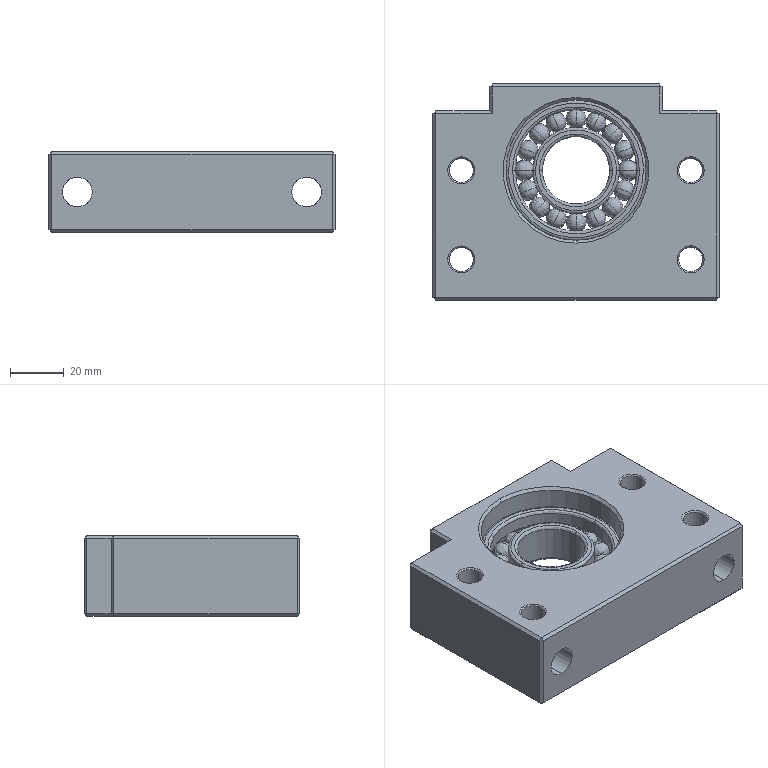Part | SolidWorks | features BaseBody 19 | 19 solids | 166 faces | box 106 x 80 x 30 mm | volume 171843 mm3 | spline 54 | plane 50 | cylinder 38 | cone 24 | commonest cylinder face diameters 9 x16 11 x4 17 x4 32 x4 45 x4 52 x4